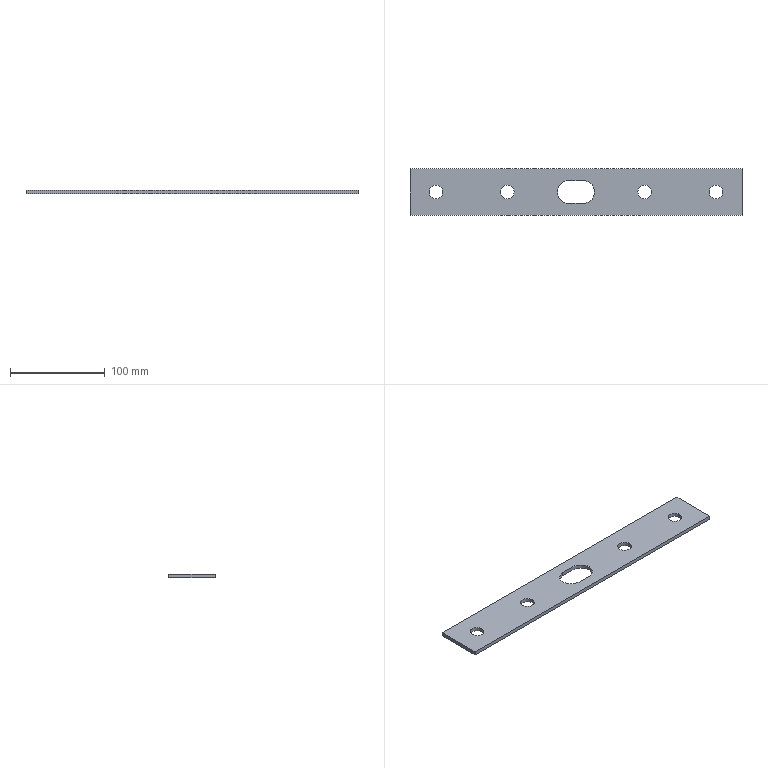Part | 1 solid | 19 faces | box 350 x 49 x 4 mm | volume 62708 mm3 | cylinder 11 | plane 8 | commonest cylinder face diameters 14.5 x8 24 x3
STEP:
#1=CARTESIAN_POINT('',(-79.75,0.,-4.));
#2=VERTEX_POINT('',#1);
#3=CARTESIAN_POINT('',(-65.25,0.,-4.));
#4=VERTEX_POINT('',#3);
#5=CARTESIAN_POINT('',(-72.5,0.,-4.));
#6=DIRECTION('',(0.,0.,1.));
#7=DIRECTION('',(1.,0.,0.));
#8=AXIS2_PLACEMENT_3D('',#5,#6,#7);
#9=CIRCLE('',#8,7.25);
#10=EDGE_CURVE('',#2,#4,#9,.T.);
#11=ORIENTED_EDGE('',*,*,#10,.F.);
#12=CARTESIAN_POINT('',(-79.75,0.,0.));
#13=VERTEX_POINT('',#12);
#14=CARTESIAN_POINT('',(-79.75,0.,-10.));
#15=DIRECTION('',(0.,0.,1.));
#16=VECTOR('',#15,1000.);
#17=LINE('',#14,#16);
#18=EDGE_CURVE('',#2,#13,#17,.T.);
#19=ORIENTED_EDGE('',*,*,#18,.T.);
#20=CARTESIAN_POINT('',(-65.25,0.,0.));
#21=VERTEX_POINT('',#20);
#22=CARTESIAN_POINT('',(-72.5,0.,0.));
#23=DIRECTION('',(0.,0.,1.));
#24=DIRECTION('',(-1.,0.,0.));
#25=AXIS2_PLACEMENT_3D('',#22,#23,#24);
#26=CIRCLE('',#25,7.25);
#27=EDGE_CURVE('',#13,#21,#26,.T.);
#28=ORIENTED_EDGE('',*,*,#27,.T.);
#29=CARTESIAN_POINT('',(-65.25,0.,-10.));
#30=DIRECTION('',(0.,0.,1.));
#31=VECTOR('',#30,1000.);
#32=LINE('',#29,#31);
#33=EDGE_CURVE('',#4,#21,#32,.T.);
#34=ORIENTED_EDGE('',*,*,#33,.F.);
#35=EDGE_LOOP('',(#11,#19,#28,#34));
#36=FACE_OUTER_BOUND('',#35,.T.);
#37=CARTESIAN_POINT('',(-72.5,0.,-10.));
#38=DIRECTION('',(0.,0.,1.));
#39=DIRECTION('',(1.,0.,0.));
#40=AXIS2_PLACEMENT_3D('',#37,#38,#39);
#41=CYLINDRICAL_SURFACE('',#40,7.25);
#42=ADVANCED_FACE('',(#36),#41,.F.);
#43=CARTESIAN_POINT('',(140.25,0.,-4.));
#44=VERTEX_POINT('',#43);
#45=CARTESIAN_POINT('',(154.75,0.,-4.));
#46=VERTEX_POINT('',#45);
#47=CARTESIAN_POINT('',(147.5,0.,-4.));
#48=DIRECTION('',(0.,0.,1.));
#49=DIRECTION('',(1.,0.,0.));
#50=AXIS2_PLACEMENT_3D('',#47,#48,#49);
#51=CIRCLE('',#50,7.25);
#52=EDGE_CURVE('',#44,#46,#51,.T.);
#53=ORIENTED_EDGE('',*,*,#52,.F.);
#54=CARTESIAN_POINT('',(140.25,0.,0.));
#55=VERTEX_POINT('',#54);
#56=CARTESIAN_POINT('',(140.25,0.,-10.));
#57=DIRECTION('',(0.,0.,1.));
#58=VECTOR('',#57,1000.);
#59=LINE('',#56,#58);
#60=EDGE_CURVE('',#44,#55,#59,.T.);
#61=ORIENTED_EDGE('',*,*,#60,.T.);
#62=CARTESIAN_POINT('',(154.75,0.,0.));
#63=VERTEX_POINT('',#62);
#64=CARTESIAN_POINT('',(147.5,0.,0.));
#65=DIRECTION('',(0.,0.,1.));
#66=DIRECTION('',(1.,0.,0.));
#67=AXIS2_PLACEMENT_3D('',#64,#65,#66);
#68=CIRCLE('',#67,7.25);
#69=EDGE_CURVE('',#55,#63,#68,.T.);
#70=ORIENTED_EDGE('',*,*,#69,.T.);
#71=CARTESIAN_POINT('',(154.75,0.,-10.));
#72=DIRECTION('',(0.,0.,1.));
#73=VECTOR('',#72,1000.);
#74=LINE('',#71,#73);
#75=EDGE_CURVE('',#46,#63,#74,.T.);
#76=ORIENTED_EDGE('',*,*,#75,.F.);
#77=EDGE_LOOP('',(#53,#61,#70,#76));
#78=FACE_OUTER_BOUND('',#77,.T.);
#79=CARTESIAN_POINT('',(147.5,0.,-10.));
#80=DIRECTION('',(0.,0.,1.));
#81=DIRECTION('',(1.,0.,0.));
#82=AXIS2_PLACEMENT_3D('',#79,#80,#81);
#83=CYLINDRICAL_SURFACE('',#82,7.25);
#84=ADVANCED_FACE('',(#78),#83,.F.);
#85=CARTESIAN_POINT('',(-154.75,0.,-4.));
#86=VERTEX_POINT('',#85);
#87=CARTESIAN_POINT('',(-140.25,0.,-4.));
#88=VERTEX_POINT('',#87);
#89=CARTESIAN_POINT('',(-147.5,0.,-4.));
#90=DIRECTION('',(0.,0.,1.));
#91=DIRECTION('',(1.,0.,0.));
#92=AXIS2_PLACEMENT_3D('',#89,#90,#91);
#93=CIRCLE('',#92,7.25);
#94=EDGE_CURVE('',#86,#88,#93,.T.);
#95=ORIENTED_EDGE('',*,*,#94,.F.);
#96=CARTESIAN_POINT('',(-154.75,0.,0.));
#97=VERTEX_POINT('',#96);
#98=CARTESIAN_POINT('',(-154.75,0.,-10.));
#99=DIRECTION('',(0.,0.,1.));
#100=VECTOR('',#99,1000.);
#101=LINE('',#98,#100);
#102=EDGE_CURVE('',#86,#97,#101,.T.);
#103=ORIENTED_EDGE('',*,*,#102,.T.);
#104=CARTESIAN_POINT('',(-140.25,0.,0.));
#105=VERTEX_POINT('',#104);
#106=CARTESIAN_POINT('',(-147.5,0.,0.));
#107=DIRECTION('',(0.,0.,1.));
#108=DIRECTION('',(-1.,0.,0.));
#109=AXIS2_PLACEMENT_3D('',#106,#107,#108);
#110=CIRCLE('',#109,7.25);
#111=EDGE_CURVE('',#97,#105,#110,.T.);
#112=ORIENTED_EDGE('',*,*,#111,.T.);
#113=CARTESIAN_POINT('',(-140.25,0.,-10.));
#114=DIRECTION('',(0.,0.,1.));
#115=VECTOR('',#114,1000.);
#116=LINE('',#113,#115);
#117=EDGE_CURVE('',#88,#105,#116,.T.);
#118=ORIENTED_EDGE('',*,*,#117,.F.);
#119=EDGE_LOOP('',(#95,#103,#112,#118));
#120=FACE_OUTER_BOUND('',#119,.T.);
#121=CARTESIAN_POINT('',(-147.5,0.,-10.));
#122=DIRECTION('',(0.,0.,1.));
#123=DIRECTION('',(1.,0.,0.));
#124=AXIS2_PLACEMENT_3D('',#121,#122,#123);
#125=CYLINDRICAL_SURFACE('',#124,7.25);
#126=ADVANCED_FACE('',(#120),#125,.F.);
#127=CARTESIAN_POINT('',(19.5,0.,-4.));
#128=VERTEX_POINT('',#127);
#129=CARTESIAN_POINT('',(7.5,12.,-4.));
#130=VERTEX_POINT('',#129);
#131=CARTESIAN_POINT('',(7.5,0.,-4.));
#132=DIRECTION('',(0.,0.,1.));
#133=DIRECTION('',(1.,0.,0.));
#134=AXIS2_PLACEMENT_3D('',#131,#132,#133);
#135=CIRCLE('',#134,12.);
#136=EDGE_CURVE('',#128,#130,#135,.T.);
#137=ORIENTED_EDGE('',*,*,#136,.F.);
#138=CARTESIAN_POINT('',(19.5,0.,0.));
#139=VERTEX_POINT('',#138);
#140=CARTESIAN_POINT('',(19.5,0.,-10.));
#141=DIRECTION('',(0.,0.,1.));
#142=VECTOR('',#141,1000.);
#143=LINE('',#140,#142);
#144=EDGE_CURVE('',#128,#139,#143,.T.);
#145=ORIENTED_EDGE('',*,*,#144,.T.);
#146=CARTESIAN_POINT('',(7.5,12.,0.));
#147=VERTEX_POINT('',#146);
#148=CARTESIAN_POINT('',(7.5,0.,0.));
#149=DIRECTION('',(0.,0.,1.));
#150=DIRECTION('',(1.,0.,0.));
#151=AXIS2_PLACEMENT_3D('',#148,#149,#150);
#152=CIRCLE('',#151,12.);
#153=EDGE_CURVE('',#139,#147,#152,.T.);
#154=ORIENTED_EDGE('',*,*,#153,.T.);
#155=CARTESIAN_POINT('',(7.5,12.,-10.));
#156=DIRECTION('',(0.,0.,1.));
#157=VECTOR('',#156,1000.);
#158=LINE('',#155,#157);
#159=EDGE_CURVE('',#130,#147,#158,.T.);
#160=ORIENTED_EDGE('',*,*,#159,.F.);
#161=EDGE_LOOP('',(#137,#145,#154,#160));
#162=FACE_OUTER_BOUND('',#161,.T.);
#163=CARTESIAN_POINT('',(7.5,0.,-10.));
#164=DIRECTION('',(0.,0.,1.));
#165=DIRECTION('',(1.,0.,0.));
#166=AXIS2_PLACEMENT_3D('',#163,#164,#165);
#167=CYLINDRICAL_SURFACE('',#166,12.);
#168=ADVANCED_FACE('',(#162),#167,.F.);
#169=CARTESIAN_POINT('',(65.25,0.,-4.));
#170=VERTEX_POINT('',#169);
#171=CARTESIAN_POINT('',(79.75,0.,-4.));
#172=VERTEX_POINT('',#171);
#173=CARTESIAN_POINT('',(72.5,0.,-4.));
#174=DIRECTION('',(0.,0.,1.));
#175=DIRECTION('',(1.,0.,0.));
#176=AXIS2_PLACEMENT_3D('',#173,#174,#175);
#177=CIRCLE('',#176,7.25);
#178=EDGE_CURVE('',#170,#172,#177,.T.);
#179=ORIENTED_EDGE('',*,*,#178,.F.);
#180=CARTESIAN_POINT('',(65.25,0.,0.));
#181=VERTEX_POINT('',#180);
#182=CARTESIAN_POINT('',(65.25,0.,-10.));
#183=DIRECTION('',(0.,0.,1.));
#184=VECTOR('',#183,1000.);
#185=LINE('',#182,#184);
#186=EDGE_CURVE('',#170,#181,#185,.T.);
#187=ORIENTED_EDGE('',*,*,#186,.T.);
#188=CARTESIAN_POINT('',(79.75,0.,0.));
#189=VERTEX_POINT('',#188);
#190=CARTESIAN_POINT('',(72.5,0.,0.));
#191=DIRECTION('',(0.,0.,1.));
#192=DIRECTION('',(1.,0.,0.));
#193=AXIS2_PLACEMENT_3D('',#190,#191,#192);
#194=CIRCLE('',#193,7.25);
#195=EDGE_CURVE('',#181,#189,#194,.T.);
#196=ORIENTED_EDGE('',*,*,#195,.T.);
#197=CARTESIAN_POINT('',(79.75,0.,-10.));
#198=DIRECTION('',(0.,0.,1.));
#199=VECTOR('',#198,1000.);
#200=LINE('',#197,#199);
#201=EDGE_CURVE('',#172,#189,#200,.T.);
#202=ORIENTED_EDGE('',*,*,#201,.F.);
#203=EDGE_LOOP('',(#179,#187,#196,#202));
#204=FACE_OUTER_BOUND('',#203,.T.);
#205=CARTESIAN_POINT('',(72.5,0.,-10.));
#206=DIRECTION('',(0.,0.,1.));
#207=DIRECTION('',(1.,0.,0.));
#208=AXIS2_PLACEMENT_3D('',#205,#206,#207);
#209=CYLINDRICAL_SURFACE('',#208,7.25);
#210=ADVANCED_FACE('',(#204),#209,.F.);
#211=CARTESIAN_POINT('',(175.,-24.5,0.));
#212=VERTEX_POINT('',#211);
#213=CARTESIAN_POINT('',(175.,24.5,0.));
#214=VERTEX_POINT('',#213);
#215=CARTESIAN_POINT('',(175.,24.5,0.));
#216=DIRECTION('',(0.,1.,0.));
#217=VECTOR('',#216,1000.);
#218=LINE('',#215,#217);
#219=EDGE_CURVE('',#212,#214,#218,.T.);
#220=ORIENTED_EDGE('',*,*,#219,.F.);
#221=CARTESIAN_POINT('',(175.,-24.5,-4.));
#222=VERTEX_POINT('',#221);
#223=CARTESIAN_POINT('',(175.,-24.5,-4.));
#224=DIRECTION('',(0.,0.,1.));
#225=VECTOR('',#224,1000.);
#226=LINE('',#223,#225);
#227=EDGE_CURVE('',#222,#212,#226,.T.);
#228=ORIENTED_EDGE('',*,*,#227,.F.);
#229=CARTESIAN_POINT('',(175.,24.5,-4.));
#230=VERTEX_POINT('',#229);
#231=CARTESIAN_POINT('',(175.,24.5,-4.));
#232=DIRECTION('',(0.,1.,0.));
#233=VECTOR('',#232,1000.);
#234=LINE('',#231,#233);
#235=EDGE_CURVE('',#222,#230,#234,.T.);
#236=ORIENTED_EDGE('',*,*,#235,.T.);
#237=CARTESIAN_POINT('',(175.,24.5,-4.));
#238=DIRECTION('',(0.,0.,1.));
#239=VECTOR('',#238,1000.);
#240=LINE('',#237,#239);
#241=EDGE_CURVE('',#230,#214,#240,.T.);
#242=ORIENTED_EDGE('',*,*,#241,.T.);
#243=EDGE_LOOP('',(#220,#228,#236,#242));
#244=FACE_OUTER_BOUND('',#243,.T.);
#245=CARTESIAN_POINT('',(175.,24.5,-4.));
#246=DIRECTION('',(1.,0.,0.));
#247=DIRECTION('',(0.,0.,-1.));
#248=AXIS2_PLACEMENT_3D('',#245,#246,#247);
#249=PLANE('',#248);
#250=ADVANCED_FACE('',(#244),#249,.T.);
#251=CARTESIAN_POINT('',(-175.,-24.5,0.));
#252=VERTEX_POINT('',#251);
#253=CARTESIAN_POINT('',(-175.,-24.5,0.));
#254=DIRECTION('',(1.,0.,0.));
#255=VECTOR('',#254,1000.);
#256=LINE('',#253,#255);
#257=EDGE_CURVE('',#252,#212,#256,.T.);
#258=ORIENTED_EDGE('',*,*,#257,.F.);
#259=CARTESIAN_POINT('',(-175.,-24.5,-4.));
#260=VERTEX_POINT('',#259);
#261=CARTESIAN_POINT('',(-175.,-24.5,-4.));
#262=DIRECTION('',(0.,0.,1.));
#263=VECTOR('',#262,1000.);
#264=LINE('',#261,#263);
#265=EDGE_CURVE('',#260,#252,#264,.T.);
#266=ORIENTED_EDGE('',*,*,#265,.F.);
#267=CARTESIAN_POINT('',(-175.,-24.5,-4.));
#268=DIRECTION('',(1.,0.,0.));
#269=VECTOR('',#268,1000.);
#270=LINE('',#267,#269);
#271=EDGE_CURVE('',#260,#222,#270,.T.);
#272=ORIENTED_EDGE('',*,*,#271,.T.);
#273=ORIENTED_EDGE('',*,*,#227,.T.);
#274=EDGE_LOOP('',(#258,#266,#272,#273));
#275=FACE_OUTER_BOUND('',#274,.T.);
#276=CARTESIAN_POINT('',(-175.,-24.5,-4.));
#277=DIRECTION('',(0.,-1.,0.));
#278=DIRECTION('',(0.,0.,-1.));
#279=AXIS2_PLACEMENT_3D('',#276,#277,#278);
#280=PLANE('',#279);
#281=ADVANCED_FACE('',(#275),#280,.T.);
#282=CARTESIAN_POINT('',(-175.,24.5,0.));
#283=VERTEX_POINT('',#282);
#284=CARTESIAN_POINT('',(-175.,24.5,0.));
#285=DIRECTION('',(0.,-1.,0.));
#286=VECTOR('',#285,1000.);
#287=LINE('',#284,#286);
#288=EDGE_CURVE('',#283,#252,#287,.T.);
#289=ORIENTED_EDGE('',*,*,#288,.F.);
#290=CARTESIAN_POINT('',(-175.,24.5,-4.));
#291=VERTEX_POINT('',#290);
#292=CARTESIAN_POINT('',(-175.,24.5,-4.));
#293=DIRECTION('',(0.,0.,1.));
#294=VECTOR('',#293,1000.);
#295=LINE('',#292,#294);
#296=EDGE_CURVE('',#291,#283,#295,.T.);
#297=ORIENTED_EDGE('',*,*,#296,.F.);
#298=CARTESIAN_POINT('',(-175.,24.5,-4.));
#299=DIRECTION('',(0.,-1.,0.));
#300=VECTOR('',#299,1000.);
#301=LINE('',#298,#300);
#302=EDGE_CURVE('',#291,#260,#301,.T.);
#303=ORIENTED_EDGE('',*,*,#302,.T.);
#304=ORIENTED_EDGE('',*,*,#265,.T.);
#305=EDGE_LOOP('',(#289,#297,#303,#304));
#306=FACE_OUTER_BOUND('',#305,.T.);
#307=CARTESIAN_POINT('',(-175.,24.5,-4.));
#308=DIRECTION('',(-1.,0.,0.));
#309=DIRECTION('',(0.,0.,1.));
#310=AXIS2_PLACEMENT_3D('',#307,#308,#309);
#311=PLANE('',#310);
#312=ADVANCED_FACE('',(#306),#311,.T.);
#313=CARTESIAN_POINT('',(-175.,24.5,0.));
#314=DIRECTION('',(-1.,0.,0.));
#315=VECTOR('',#314,1000.);
#316=LINE('',#313,#315);
#317=EDGE_CURVE('',#214,#283,#316,.T.);
#318=ORIENTED_EDGE('',*,*,#317,.F.);
#319=ORIENTED_EDGE('',*,*,#241,.F.);
#320=CARTESIAN_POINT('',(-175.,24.5,-4.));
#321=DIRECTION('',(-1.,0.,0.));
#322=VECTOR('',#321,1000.);
#323=LINE('',#320,#322);
#324=EDGE_CURVE('',#230,#291,#323,.T.);
#325=ORIENTED_EDGE('',*,*,#324,.T.);
#326=ORIENTED_EDGE('',*,*,#296,.T.);
#327=EDGE_LOOP('',(#318,#319,#325,#326));
#328=FACE_OUTER_BOUND('',#327,.T.);
#329=CARTESIAN_POINT('',(-175.,24.5,-4.));
#330=DIRECTION('',(0.,1.,0.));
#331=DIRECTION('',(0.,0.,1.));
#332=AXIS2_PLACEMENT_3D('',#329,#330,#331);
#333=PLANE('',#332);
#334=ADVANCED_FACE('',(#328),#333,.T.);
#335=CARTESIAN_POINT('',(-72.5,0.,-4.));
#336=DIRECTION('',(0.,0.,1.));
#337=DIRECTION('',(1.,0.,0.));
#338=AXIS2_PLACEMENT_3D('',#335,#336,#337);
#339=CIRCLE('',#338,7.25);
#340=EDGE_CURVE('',#4,#2,#339,.T.);
#341=ORIENTED_EDGE('',*,*,#340,.T.);
#342=ORIENTED_EDGE('',*,*,#10,.T.);
#343=EDGE_LOOP('',(#341,#342));
#344=FACE_BOUND('',#343,.T.);
#345=CARTESIAN_POINT('',(147.5,0.,-4.));
#346=DIRECTION('',(0.,0.,1.));
#347=DIRECTION('',(1.,0.,0.));
#348=AXIS2_PLACEMENT_3D('',#345,#346,#347);
#349=CIRCLE('',#348,7.25);
#350=EDGE_CURVE('',#46,#44,#349,.T.);
#351=ORIENTED_EDGE('',*,*,#350,.T.);
#352=ORIENTED_EDGE('',*,*,#52,.T.);
#353=EDGE_LOOP('',(#351,#352));
#354=FACE_BOUND('',#353,.T.);
#355=CARTESIAN_POINT('',(-147.5,0.,-4.));
#356=DIRECTION('',(0.,0.,1.));
#357=DIRECTION('',(1.,0.,0.));
#358=AXIS2_PLACEMENT_3D('',#355,#356,#357);
#359=CIRCLE('',#358,7.25);
#360=EDGE_CURVE('',#88,#86,#359,.T.);
#361=ORIENTED_EDGE('',*,*,#360,.T.);
#362=ORIENTED_EDGE('',*,*,#94,.T.);
#363=EDGE_LOOP('',(#361,#362));
#364=FACE_BOUND('',#363,.T.);
#365=CARTESIAN_POINT('',(-7.5,12.,-4.));
#366=VERTEX_POINT('',#365);
#367=CARTESIAN_POINT('',(0.,12.,-4.));
#368=DIRECTION('',(-1.,0.,0.));
#369=VECTOR('',#368,1000.);
#370=LINE('',#367,#369);
#371=EDGE_CURVE('',#130,#366,#370,.T.);
#372=ORIENTED_EDGE('',*,*,#371,.T.);
#373=CARTESIAN_POINT('',(-7.5,-12.,-4.));
#374=VERTEX_POINT('',#373);
#375=CARTESIAN_POINT('',(-7.5,0.,-4.));
#376=DIRECTION('',(0.,0.,1.));
#377=DIRECTION('',(1.,0.,0.));
#378=AXIS2_PLACEMENT_3D('',#375,#376,#377);
#379=CIRCLE('',#378,12.);
#380=EDGE_CURVE('',#366,#374,#379,.T.);
#381=ORIENTED_EDGE('',*,*,#380,.T.);
#382=CARTESIAN_POINT('',(7.5,-12.,-4.));
#383=VERTEX_POINT('',#382);
#384=CARTESIAN_POINT('',(0.,-12.,-4.));
#385=DIRECTION('',(1.,0.,0.));
#386=VECTOR('',#385,1000.);
#387=LINE('',#384,#386);
#388=EDGE_CURVE('',#374,#383,#387,.T.);
#389=ORIENTED_EDGE('',*,*,#388,.T.);
#390=CARTESIAN_POINT('',(7.5,0.,-4.));
#391=DIRECTION('',(0.,0.,1.));
#392=DIRECTION('',(1.,0.,0.));
#393=AXIS2_PLACEMENT_3D('',#390,#391,#392);
#394=CIRCLE('',#393,12.);
#395=EDGE_CURVE('',#383,#128,#394,.T.);
#396=ORIENTED_EDGE('',*,*,#395,.T.);
#397=ORIENTED_EDGE('',*,*,#136,.T.);
#398=EDGE_LOOP('',(#372,#381,#389,#396,#397));
#399=FACE_BOUND('',#398,.T.);
#400=CARTESIAN_POINT('',(72.5,0.,-4.));
#401=DIRECTION('',(0.,0.,1.));
#402=DIRECTION('',(1.,0.,0.));
#403=AXIS2_PLACEMENT_3D('',#400,#401,#402);
#404=CIRCLE('',#403,7.25);
#405=EDGE_CURVE('',#172,#170,#404,.T.);
#406=ORIENTED_EDGE('',*,*,#405,.T.);
#407=ORIENTED_EDGE('',*,*,#178,.T.);
#408=EDGE_LOOP('',(#406,#407));
#409=FACE_BOUND('',#408,.T.);
#410=ORIENTED_EDGE('',*,*,#235,.F.);
#411=ORIENTED_EDGE('',*,*,#271,.F.);
#412=ORIENTED_EDGE('',*,*,#302,.F.);
#413=ORIENTED_EDGE('',*,*,#324,.F.);
#414=EDGE_LOOP('',(#410,#411,#412,#413));
#415=FACE_OUTER_BOUND('',#414,.T.);
#416=CARTESIAN_POINT('',(0.,0.,-4.));
#417=DIRECTION('',(0.,0.,1.));
#418=DIRECTION('',(1.,0.,0.));
#419=AXIS2_PLACEMENT_3D('',#416,#417,#418);
#420=PLANE('',#419);
#421=ADVANCED_FACE('',(#344,#354,#364,#399,#409,#415),#420,.F.);
#422=CARTESIAN_POINT('',(-72.5,0.,0.));
#423=DIRECTION('',(0.,0.,1.));
#424=DIRECTION('',(-1.,0.,0.));
#425=AXIS2_PLACEMENT_3D('',#422,#423,#424);
#426=CIRCLE('',#425,7.25);
#427=EDGE_CURVE('',#21,#13,#426,.T.);
#428=ORIENTED_EDGE('',*,*,#427,.F.);
#429=ORIENTED_EDGE('',*,*,#27,.F.);
#430=EDGE_LOOP('',(#428,#429));
#431=FACE_BOUND('',#430,.T.);
#432=CARTESIAN_POINT('',(147.5,0.,0.));
#433=DIRECTION('',(0.,0.,1.));
#434=DIRECTION('',(1.,0.,0.));
#435=AXIS2_PLACEMENT_3D('',#432,#433,#434);
#436=CIRCLE('',#435,7.25);
#437=EDGE_CURVE('',#63,#55,#436,.T.);
#438=ORIENTED_EDGE('',*,*,#437,.F.);
#439=ORIENTED_EDGE('',*,*,#69,.F.);
#440=EDGE_LOOP('',(#438,#439));
#441=FACE_BOUND('',#440,.T.);
#442=CARTESIAN_POINT('',(-147.5,0.,0.));
#443=DIRECTION('',(0.,0.,1.));
#444=DIRECTION('',(-1.,0.,0.));
#445=AXIS2_PLACEMENT_3D('',#442,#443,#444);
#446=CIRCLE('',#445,7.25);
#447=EDGE_CURVE('',#105,#97,#446,.T.);
#448=ORIENTED_EDGE('',*,*,#447,.F.);
#449=ORIENTED_EDGE('',*,*,#111,.F.);
#450=EDGE_LOOP('',(#448,#449));
#451=FACE_BOUND('',#450,.T.);
#452=CARTESIAN_POINT('',(-7.5,12.,0.));
#453=VERTEX_POINT('',#452);
#454=CARTESIAN_POINT('',(-7.5,-12.,0.));
#455=VERTEX_POINT('',#454);
#456=CARTESIAN_POINT('',(-7.5,0.,0.));
#457=DIRECTION('',(0.,0.,1.));
#458=DIRECTION('',(1.,0.,0.));
#459=AXIS2_PLACEMENT_3D('',#456,#457,#458);
#460=CIRCLE('',#459,12.);
#461=EDGE_CURVE('',#453,#455,#460,.T.);
#462=ORIENTED_EDGE('',*,*,#461,.F.);
#463=CARTESIAN_POINT('',(-7.5,12.,0.));
#464=DIRECTION('',(-1.,0.,0.));
#465=VECTOR('',#464,1000.);
#466=LINE('',#463,#465);
#467=EDGE_CURVE('',#147,#453,#466,.T.);
#468=ORIENTED_EDGE('',*,*,#467,.F.);
#469=ORIENTED_EDGE('',*,*,#153,.F.);
#470=CARTESIAN_POINT('',(7.5,-12.,0.));
#471=VERTEX_POINT('',#470);
#472=CARTESIAN_POINT('',(7.5,0.,0.));
#473=DIRECTION('',(0.,0.,1.));
#474=DIRECTION('',(1.,0.,0.));
#475=AXIS2_PLACEMENT_3D('',#472,#473,#474);
#476=CIRCLE('',#475,12.);
#477=EDGE_CURVE('',#471,#139,#476,.T.);
#478=ORIENTED_EDGE('',*,*,#477,.F.);
#479=CARTESIAN_POINT('',(-7.5,-12.,0.));
#480=DIRECTION('',(1.,0.,0.));
#481=VECTOR('',#480,1000.);
#482=LINE('',#479,#481);
#483=EDGE_CURVE('',#455,#471,#482,.T.);
#484=ORIENTED_EDGE('',*,*,#483,.F.);
#485=EDGE_LOOP('',(#462,#468,#469,#478,#484));
#486=FACE_BOUND('',#485,.T.);
#487=CARTESIAN_POINT('',(72.5,0.,0.));
#488=DIRECTION('',(0.,0.,1.));
#489=DIRECTION('',(1.,0.,0.));
#490=AXIS2_PLACEMENT_3D('',#487,#488,#489);
#491=CIRCLE('',#490,7.25);
#492=EDGE_CURVE('',#189,#181,#491,.T.);
#493=ORIENTED_EDGE('',*,*,#492,.F.);
#494=ORIENTED_EDGE('',*,*,#195,.F.);
#495=EDGE_LOOP('',(#493,#494));
#496=FACE_BOUND('',#495,.T.);
#497=ORIENTED_EDGE('',*,*,#219,.T.);
#498=ORIENTED_EDGE('',*,*,#317,.T.);
#499=ORIENTED_EDGE('',*,*,#288,.T.);
#500=ORIENTED_EDGE('',*,*,#257,.T.);
#501=EDGE_LOOP('',(#497,#498,#499,#500));
#502=FACE_OUTER_BOUND('',#501,.T.);
#503=CARTESIAN_POINT('',(0.,0.,0.));
#504=DIRECTION('',(0.,0.,1.));
#505=DIRECTION('',(1.,0.,0.));
#506=AXIS2_PLACEMENT_3D('',#503,#504,#505);
#507=PLANE('',#506);
#508=ADVANCED_FACE('',(#431,#441,#451,#486,#496,#502),#507,.T.);
#509=ORIENTED_EDGE('',*,*,#186,.F.);
#510=ORIENTED_EDGE('',*,*,#405,.F.);
#511=ORIENTED_EDGE('',*,*,#201,.T.);
#512=ORIENTED_EDGE('',*,*,#492,.T.);
#513=EDGE_LOOP('',(#509,#510,#511,#512));
#514=FACE_OUTER_BOUND('',#513,.T.);
#515=CARTESIAN_POINT('',(72.5,0.,-10.));
#516=DIRECTION('',(0.,0.,1.));
#517=DIRECTION('',(1.,0.,0.));
#518=AXIS2_PLACEMENT_3D('',#515,#516,#517);
#519=CYLINDRICAL_SURFACE('',#518,7.25);
#520=ADVANCED_FACE('',(#514),#519,.F.);
#521=CARTESIAN_POINT('',(-7.5,12.,-10.));
#522=DIRECTION('',(0.,0.,1.));
#523=VECTOR('',#522,1000.);
#524=LINE('',#521,#523);
#525=EDGE_CURVE('',#366,#453,#524,.T.);
#526=ORIENTED_EDGE('',*,*,#525,.T.);
#527=ORIENTED_EDGE('',*,*,#461,.T.);
#528=CARTESIAN_POINT('',(-7.5,-12.,-10.));
#529=DIRECTION('',(0.,0.,1.));
#530=VECTOR('',#529,1000.);
#531=LINE('',#528,#530);
#532=EDGE_CURVE('',#374,#455,#531,.T.);
#533=ORIENTED_EDGE('',*,*,#532,.F.);
#534=ORIENTED_EDGE('',*,*,#380,.F.);
#535=EDGE_LOOP('',(#526,#527,#533,#534));
#536=FACE_OUTER_BOUND('',#535,.T.);
#537=CARTESIAN_POINT('',(-7.5,0.,-10.));
#538=DIRECTION('',(0.,0.,1.));
#539=DIRECTION('',(1.,0.,0.));
#540=AXIS2_PLACEMENT_3D('',#537,#538,#539);
#541=CYLINDRICAL_SURFACE('',#540,12.);
#542=ADVANCED_FACE('',(#536),#541,.F.);
#543=ORIENTED_EDGE('',*,*,#159,.T.);
#544=ORIENTED_EDGE('',*,*,#467,.T.);
#545=ORIENTED_EDGE('',*,*,#525,.F.);
#546=ORIENTED_EDGE('',*,*,#371,.F.);
#547=EDGE_LOOP('',(#543,#544,#545,#546));
#548=FACE_OUTER_BOUND('',#547,.T.);
#549=CARTESIAN_POINT('',(-7.5,12.,-10.));
#550=DIRECTION('',(0.,1.,0.));
#551=DIRECTION('',(-1.,0.,0.));
#552=AXIS2_PLACEMENT_3D('',#549,#550,#551);
#553=PLANE('',#552);
#554=ADVANCED_FACE('',(#548),#553,.F.);
#555=ORIENTED_EDGE('',*,*,#144,.F.);
#556=ORIENTED_EDGE('',*,*,#395,.F.);
#557=CARTESIAN_POINT('',(7.5,-12.,-10.));
#558=DIRECTION('',(0.,0.,1.));
#559=VECTOR('',#558,1000.);
#560=LINE('',#557,#559);
#561=EDGE_CURVE('',#383,#471,#560,.T.);
#562=ORIENTED_EDGE('',*,*,#561,.T.);
#563=ORIENTED_EDGE('',*,*,#477,.T.);
#564=EDGE_LOOP('',(#555,#556,#562,#563));
#565=FACE_OUTER_BOUND('',#564,.T.);
#566=CARTESIAN_POINT('',(7.5,0.,-10.));
#567=DIRECTION('',(0.,0.,1.));
#568=DIRECTION('',(1.,0.,0.));
#569=AXIS2_PLACEMENT_3D('',#566,#567,#568);
#570=CYLINDRICAL_SURFACE('',#569,12.);
#571=ADVANCED_FACE('',(#565),#570,.F.);
#572=ORIENTED_EDGE('',*,*,#532,.T.);
#573=ORIENTED_EDGE('',*,*,#483,.T.);
#574=ORIENTED_EDGE('',*,*,#561,.F.);
#575=ORIENTED_EDGE('',*,*,#388,.F.);
#576=EDGE_LOOP('',(#572,#573,#574,#575));
#577=FACE_OUTER_BOUND('',#576,.T.);
#578=CARTESIAN_POINT('',(-7.5,-12.,-10.));
#579=DIRECTION('',(0.,-1.,0.));
#580=DIRECTION('',(0.,0.,-1.));
#581=AXIS2_PLACEMENT_3D('',#578,#579,#580);
#582=PLANE('',#581);
#583=ADVANCED_FACE('',(#577),#582,.F.);
#584=ORIENTED_EDGE('',*,*,#102,.F.);
#585=ORIENTED_EDGE('',*,*,#360,.F.);
#586=ORIENTED_EDGE('',*,*,#117,.T.);
#587=ORIENTED_EDGE('',*,*,#447,.T.);
#588=EDGE_LOOP('',(#584,#585,#586,#587));
#589=FACE_OUTER_BOUND('',#588,.T.);
#590=CARTESIAN_POINT('',(-147.5,0.,-10.));
#591=DIRECTION('',(0.,0.,1.));
#592=DIRECTION('',(1.,0.,0.));
#593=AXIS2_PLACEMENT_3D('',#590,#591,#592);
#594=CYLINDRICAL_SURFACE('',#593,7.25);
#595=ADVANCED_FACE('',(#589),#594,.F.);
#596=ORIENTED_EDGE('',*,*,#60,.F.);
#597=ORIENTED_EDGE('',*,*,#350,.F.);
#598=ORIENTED_EDGE('',*,*,#75,.T.);
#599=ORIENTED_EDGE('',*,*,#437,.T.);
#600=EDGE_LOOP('',(#596,#597,#598,#599));
#601=FACE_OUTER_BOUND('',#600,.T.);
#602=CARTESIAN_POINT('',(147.5,0.,-10.));
#603=DIRECTION('',(0.,0.,1.));
#604=DIRECTION('',(1.,0.,0.));
#605=AXIS2_PLACEMENT_3D('',#602,#603,#604);
#606=CYLINDRICAL_SURFACE('',#605,7.25);
#607=ADVANCED_FACE('',(#601),#606,.F.);
#608=ORIENTED_EDGE('',*,*,#18,.F.);
#609=ORIENTED_EDGE('',*,*,#340,.F.);
#610=ORIENTED_EDGE('',*,*,#33,.T.);
#611=ORIENTED_EDGE('',*,*,#427,.T.);
#612=EDGE_LOOP('',(#608,#609,#610,#611));
#613=FACE_OUTER_BOUND('',#612,.T.);
#614=CARTESIAN_POINT('',(-72.5,0.,-10.));
#615=DIRECTION('',(0.,0.,1.));
#616=DIRECTION('',(1.,0.,0.));
#617=AXIS2_PLACEMENT_3D('',#614,#615,#616);
#618=CYLINDRICAL_SURFACE('',#617,7.25);
#619=ADVANCED_FACE('',(#613),#618,.F.);
#620=CLOSED_SHELL('',(#42,#84,#126,#168,#210,#250,#281,#312,#334,#421,#508,#520,#542,#554,#571,#583,#595,#607,#619));
#621=MANIFOLD_SOLID_BREP('',#620);
#622=CARTESIAN_POINT('',(0.,0.,0.));
#623=DIRECTION('',(0.,0.,1.));
#624=DIRECTION('',(1.,0.,0.));
#625=AXIS2_PLACEMENT_3D('',#622,#623,#624);
#626=(LENGTH_UNIT()NAMED_UNIT(*)SI_UNIT(.MILLI.,.METRE.));
#627=UNCERTAINTY_MEASURE_WITH_UNIT(LENGTH_MEASURE(0.00001),#626,'','');
#628=(NAMED_UNIT(*)PLANE_ANGLE_UNIT()SI_UNIT($,.RADIAN.));
#629=(NAMED_UNIT(*)SI_UNIT($,.STERADIAN.)SOLID_ANGLE_UNIT());
#630=(GEOMETRIC_REPRESENTATION_CONTEXT(3)GLOBAL_UNCERTAINTY_ASSIGNED_CONTEXT((#627))GLOBAL_UNIT_ASSIGNED_CONTEXT((#626,#628,#629))REPRESENTATION_CONTEXT('',''));
#631=ADVANCED_BREP_SHAPE_REPRESENTATION('',(#621,#625),#630);